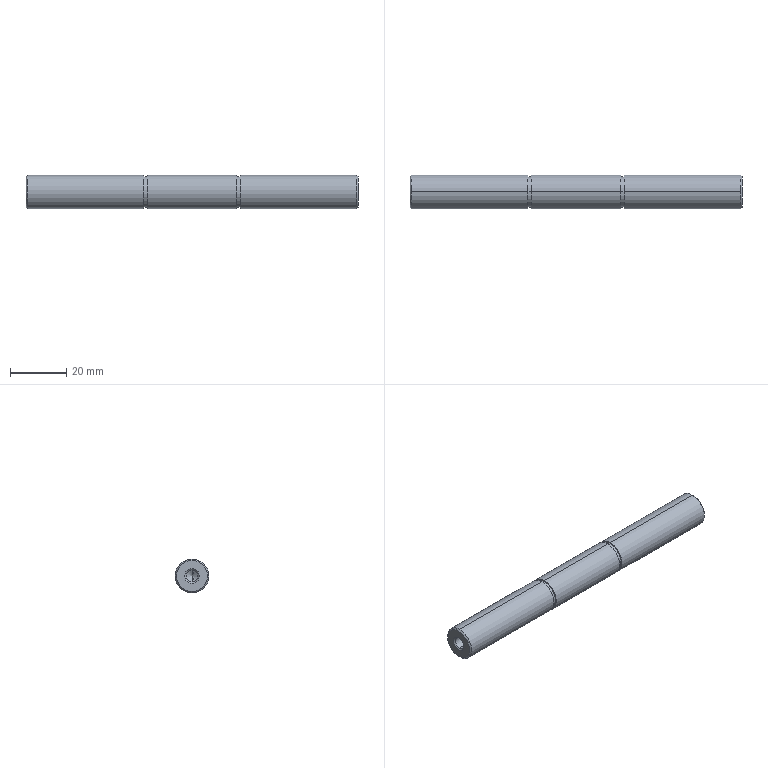Part | SolidWorks | features BaseBody 1 | 1 solid | 32 faces | box 118 x 12 x 12 mm | volume 12890 mm3 | cylinder 14 | cone 12 | plane 6 | commonest cylinder face diameters 12 x6 4.2 x4 11 x4
STEP:
#1=CARTESIAN_POINT('',(41.9,0.,6.));
#2=VERTEX_POINT('',#1);
#3=CARTESIAN_POINT('',(41.9,0.,-6.));
#4=VERTEX_POINT('',#3);
#5=CARTESIAN_POINT('',(41.9,0.,0.));
#6=DIRECTION('',(-1.,0.,0.));
#7=DIRECTION('',(0.,0.,1.));
#8=AXIS2_PLACEMENT_3D('',#5,#6,#7);
#9=CIRCLE('',#8,6.);
#10=EDGE_CURVE('',#2,#4,#9,.T.);
#11=ORIENTED_EDGE('',*,*,#10,.T.);
#12=CARTESIAN_POINT('',(0.5,0.,-6.));
#13=VERTEX_POINT('',#12);
#14=CARTESIAN_POINT('',(118.,0.,-6.));
#15=DIRECTION('',(-1.,0.,0.));
#16=VECTOR('',#15,1000.);
#17=LINE('',#14,#16);
#18=EDGE_CURVE('',#4,#13,#17,.T.);
#19=ORIENTED_EDGE('',*,*,#18,.T.);
#20=CARTESIAN_POINT('',(0.5,0.,6.));
#21=VERTEX_POINT('',#20);
#22=CARTESIAN_POINT('',(0.5,0.,0.));
#23=DIRECTION('',(1.,0.,0.));
#24=DIRECTION('',(0.,0.,-1.));
#25=AXIS2_PLACEMENT_3D('',#22,#23,#24);
#26=CIRCLE('',#25,6.);
#27=EDGE_CURVE('',#13,#21,#26,.T.);
#28=ORIENTED_EDGE('',*,*,#27,.T.);
#29=CARTESIAN_POINT('',(118.,0.,6.));
#30=DIRECTION('',(-1.,0.,0.));
#31=VECTOR('',#30,1000.);
#32=LINE('',#29,#31);
#33=EDGE_CURVE('',#2,#21,#32,.T.);
#34=ORIENTED_EDGE('',*,*,#33,.F.);
#35=EDGE_LOOP('',(#11,#19,#28,#34));
#36=FACE_OUTER_BOUND('',#35,.T.);
#37=CARTESIAN_POINT('',(118.,0.,0.));
#38=DIRECTION('',(-1.,0.,0.));
#39=DIRECTION('',(0.,0.,1.));
#40=AXIS2_PLACEMENT_3D('',#37,#38,#39);
#41=CYLINDRICAL_SURFACE('',#40,6.);
#42=ADVANCED_FACE('',(#36),#41,.T.);
#43=CARTESIAN_POINT('',(0.,0.,5.5));
#44=VERTEX_POINT('',#43);
#45=CARTESIAN_POINT('',(0.,0.,-5.5));
#46=VERTEX_POINT('',#45);
#47=CARTESIAN_POINT('',(0.,0.,0.));
#48=DIRECTION('',(-1.,0.,0.));
#49=DIRECTION('',(0.,0.,-1.));
#50=AXIS2_PLACEMENT_3D('',#47,#48,#49);
#51=CIRCLE('',#50,5.5);
#52=EDGE_CURVE('',#44,#46,#51,.T.);
#53=ORIENTED_EDGE('',*,*,#52,.F.);
#54=CARTESIAN_POINT('',(0.5,0.,6.));
#55=DIRECTION('',(0.7071,0.,0.7071));
#56=VECTOR('',#55,1000.);
#57=LINE('',#54,#56);
#58=EDGE_CURVE('',#44,#21,#57,.T.);
#59=ORIENTED_EDGE('',*,*,#58,.T.);
#60=ORIENTED_EDGE('',*,*,#27,.F.);
#61=CARTESIAN_POINT('',(0.5,0.,-6.));
#62=DIRECTION('',(0.7071,0.,-0.7071));
#63=VECTOR('',#62,1000.);
#64=LINE('',#61,#63);
#65=EDGE_CURVE('',#46,#13,#64,.T.);
#66=ORIENTED_EDGE('',*,*,#65,.F.);
#67=EDGE_LOOP('',(#53,#59,#60,#66));
#68=FACE_OUTER_BOUND('',#67,.T.);
#69=CARTESIAN_POINT('',(0.5,0.,0.));
#70=DIRECTION('',(1.,0.,0.));
#71=DIRECTION('',(0.,0.,-1.));
#72=AXIS2_PLACEMENT_3D('',#69,#70,#71);
#73=CONICAL_SURFACE('',#72,6.,0.7854);
#74=ADVANCED_FACE('',(#68),#73,.T.);
#75=CARTESIAN_POINT('',(0.5,0.,-2.1));
#76=VERTEX_POINT('',#75);
#77=CARTESIAN_POINT('',(0.5,0.,2.1));
#78=VERTEX_POINT('',#77);
#79=CARTESIAN_POINT('',(0.5,0.,0.));
#80=DIRECTION('',(-1.,0.,0.));
#81=DIRECTION('',(0.,0.,-1.));
#82=AXIS2_PLACEMENT_3D('',#79,#80,#81);
#83=CIRCLE('',#82,2.1);
#84=EDGE_CURVE('',#76,#78,#83,.T.);
#85=ORIENTED_EDGE('',*,*,#84,.F.);
#86=CARTESIAN_POINT('',(0.,0.,-2.6));
#87=VERTEX_POINT('',#86);
#88=CARTESIAN_POINT('',(0.5,0.,-2.1));
#89=DIRECTION('',(-0.7071,0.,-0.7071));
#90=VECTOR('',#89,1000.);
#91=LINE('',#88,#90);
#92=EDGE_CURVE('',#76,#87,#91,.T.);
#93=ORIENTED_EDGE('',*,*,#92,.T.);
#94=CARTESIAN_POINT('',(0.,0.,2.6));
#95=VERTEX_POINT('',#94);
#96=CARTESIAN_POINT('',(0.,0.,0.));
#97=DIRECTION('',(1.,0.,0.));
#98=DIRECTION('',(0.,0.,-1.));
#99=AXIS2_PLACEMENT_3D('',#96,#97,#98);
#100=CIRCLE('',#99,2.6);
#101=EDGE_CURVE('',#95,#87,#100,.T.);
#102=ORIENTED_EDGE('',*,*,#101,.F.);
#103=CARTESIAN_POINT('',(0.5,0.,2.1));
#104=DIRECTION('',(-0.7071,0.,0.7071));
#105=VECTOR('',#104,1000.);
#106=LINE('',#103,#105);
#107=EDGE_CURVE('',#78,#95,#106,.T.);
#108=ORIENTED_EDGE('',*,*,#107,.F.);
#109=EDGE_LOOP('',(#85,#93,#102,#108));
#110=FACE_OUTER_BOUND('',#109,.T.);
#111=CARTESIAN_POINT('',(0.5,0.,0.));
#112=DIRECTION('',(-1.,0.,0.));
#113=DIRECTION('',(0.,0.,1.));
#114=AXIS2_PLACEMENT_3D('',#111,#112,#113);
#115=CONICAL_SURFACE('',#114,2.1,0.7854);
#116=ADVANCED_FACE('',(#110),#115,.F.);
#117=CARTESIAN_POINT('',(14.,0.,-2.1));
#118=VERTEX_POINT('',#117);
#119=CARTESIAN_POINT('',(14.,0.,2.1));
#120=VERTEX_POINT('',#119);
#121=CARTESIAN_POINT('',(14.,0.,0.));
#122=DIRECTION('',(-1.,0.,0.));
#123=DIRECTION('',(0.,0.,1.));
#124=AXIS2_PLACEMENT_3D('',#121,#122,#123);
#125=CIRCLE('',#124,2.1);
#126=EDGE_CURVE('',#118,#120,#125,.T.);
#127=ORIENTED_EDGE('',*,*,#126,.F.);
#128=CARTESIAN_POINT('',(0.,0.,-2.1));
#129=DIRECTION('',(-1.,0.,0.));
#130=VECTOR('',#129,1000.);
#131=LINE('',#128,#130);
#132=EDGE_CURVE('',#118,#76,#131,.T.);
#133=ORIENTED_EDGE('',*,*,#132,.T.);
#134=ORIENTED_EDGE('',*,*,#84,.T.);
#135=CARTESIAN_POINT('',(0.,0.,2.1));
#136=DIRECTION('',(-1.,0.,0.));
#137=VECTOR('',#136,1000.);
#138=LINE('',#135,#137);
#139=EDGE_CURVE('',#120,#78,#138,.T.);
#140=ORIENTED_EDGE('',*,*,#139,.F.);
#141=EDGE_LOOP('',(#127,#133,#134,#140));
#142=FACE_OUTER_BOUND('',#141,.T.);
#143=CARTESIAN_POINT('',(0.,0.,0.));
#144=DIRECTION('',(-1.,0.,0.));
#145=DIRECTION('',(0.,0.,1.));
#146=AXIS2_PLACEMENT_3D('',#143,#144,#145);
#147=CYLINDRICAL_SURFACE('',#146,2.1);
#148=ADVANCED_FACE('',(#142),#147,.F.);
#149=CARTESIAN_POINT('',(15.262,0.,0.));
#150=VERTEX_POINT('',#149);
#151=CARTESIAN_POINT('',(14.,0.,2.1));
#152=DIRECTION('',(-0.515,0.,0.8572));
#153=VECTOR('',#152,1000.);
#154=LINE('',#151,#153);
#155=EDGE_CURVE('',#150,#120,#154,.T.);
#156=ORIENTED_EDGE('',*,*,#155,.F.);
#157=CARTESIAN_POINT('',(14.,0.,-2.1));
#158=DIRECTION('',(-0.515,0.,-0.8572));
#159=VECTOR('',#158,1000.);
#160=LINE('',#157,#159);
#161=EDGE_CURVE('',#150,#118,#160,.T.);
#162=ORIENTED_EDGE('',*,*,#161,.T.);
#163=ORIENTED_EDGE('',*,*,#126,.T.);
#164=EDGE_LOOP('',(#156,#162,#163));
#165=FACE_OUTER_BOUND('',#164,.T.);
#166=CARTESIAN_POINT('',(14.,0.,0.));
#167=DIRECTION('',(-1.,0.,0.));
#168=DIRECTION('',(0.,0.,1.));
#169=AXIS2_PLACEMENT_3D('',#166,#167,#168);
#170=CONICAL_SURFACE('',#169,2.1,1.03);
#171=ADVANCED_FACE('',(#165),#170,.F.);
#172=CARTESIAN_POINT('',(43.1,0.,5.5));
#173=VERTEX_POINT('',#172);
#174=CARTESIAN_POINT('',(43.1,0.,-5.5));
#175=VERTEX_POINT('',#174);
#176=CARTESIAN_POINT('',(43.1,0.,0.));
#177=DIRECTION('',(-1.,0.,0.));
#178=DIRECTION('',(0.,0.,1.));
#179=AXIS2_PLACEMENT_3D('',#176,#177,#178);
#180=CIRCLE('',#179,5.5);
#181=EDGE_CURVE('',#173,#175,#180,.T.);
#182=ORIENTED_EDGE('',*,*,#181,.T.);
#183=CARTESIAN_POINT('',(41.9,0.,-5.5));
#184=VERTEX_POINT('',#183);
#185=CARTESIAN_POINT('',(0.,0.,-5.5));
#186=DIRECTION('',(-1.,0.,0.));
#187=VECTOR('',#186,1000.);
#188=LINE('',#185,#187);
#189=EDGE_CURVE('',#175,#184,#188,.T.);
#190=ORIENTED_EDGE('',*,*,#189,.T.);
#191=CARTESIAN_POINT('',(41.9,0.,5.5));
#192=VERTEX_POINT('',#191);
#193=CARTESIAN_POINT('',(41.9,0.,0.));
#194=DIRECTION('',(-1.,0.,0.));
#195=DIRECTION('',(0.,0.,1.));
#196=AXIS2_PLACEMENT_3D('',#193,#194,#195);
#197=CIRCLE('',#196,5.5);
#198=EDGE_CURVE('',#192,#184,#197,.T.);
#199=ORIENTED_EDGE('',*,*,#198,.F.);
#200=CARTESIAN_POINT('',(0.,0.,5.5));
#201=DIRECTION('',(-1.,0.,0.));
#202=VECTOR('',#201,1000.);
#203=LINE('',#200,#202);
#204=EDGE_CURVE('',#173,#192,#203,.T.);
#205=ORIENTED_EDGE('',*,*,#204,.F.);
#206=EDGE_LOOP('',(#182,#190,#199,#205));
#207=FACE_OUTER_BOUND('',#206,.T.);
#208=CARTESIAN_POINT('',(0.,0.,0.));
#209=DIRECTION('',(-1.,0.,0.));
#210=DIRECTION('',(0.,0.,1.));
#211=AXIS2_PLACEMENT_3D('',#208,#209,#210);
#212=CYLINDRICAL_SURFACE('',#211,5.5);
#213=ADVANCED_FACE('',(#207),#212,.T.);
#214=CARTESIAN_POINT('',(76.1,0.,5.5));
#215=VERTEX_POINT('',#214);
#216=CARTESIAN_POINT('',(76.1,0.,-5.5));
#217=VERTEX_POINT('',#216);
#218=CARTESIAN_POINT('',(76.1,0.,0.));
#219=DIRECTION('',(-1.,0.,0.));
#220=DIRECTION('',(0.,0.,1.));
#221=AXIS2_PLACEMENT_3D('',#218,#219,#220);
#222=CIRCLE('',#221,5.5);
#223=EDGE_CURVE('',#215,#217,#222,.T.);
#224=ORIENTED_EDGE('',*,*,#223,.T.);
#225=CARTESIAN_POINT('',(74.9,0.,-5.5));
#226=VERTEX_POINT('',#225);
#227=CARTESIAN_POINT('',(0.,0.,-5.5));
#228=DIRECTION('',(-1.,0.,0.));
#229=VECTOR('',#228,1000.);
#230=LINE('',#227,#229);
#231=EDGE_CURVE('',#217,#226,#230,.T.);
#232=ORIENTED_EDGE('',*,*,#231,.T.);
#233=CARTESIAN_POINT('',(74.9,0.,5.5));
#234=VERTEX_POINT('',#233);
#235=CARTESIAN_POINT('',(74.9,0.,0.));
#236=DIRECTION('',(-1.,0.,0.));
#237=DIRECTION('',(0.,0.,1.));
#238=AXIS2_PLACEMENT_3D('',#235,#236,#237);
#239=CIRCLE('',#238,5.5);
#240=EDGE_CURVE('',#234,#226,#239,.T.);
#241=ORIENTED_EDGE('',*,*,#240,.F.);
#242=CARTESIAN_POINT('',(0.,0.,5.5));
#243=DIRECTION('',(-1.,0.,0.));
#244=VECTOR('',#243,1000.);
#245=LINE('',#242,#244);
#246=EDGE_CURVE('',#215,#234,#245,.T.);
#247=ORIENTED_EDGE('',*,*,#246,.F.);
#248=EDGE_LOOP('',(#224,#232,#241,#247));
#249=FACE_OUTER_BOUND('',#248,.T.);
#250=CARTESIAN_POINT('',(0.,0.,0.));
#251=DIRECTION('',(-1.,0.,0.));
#252=DIRECTION('',(0.,0.,1.));
#253=AXIS2_PLACEMENT_3D('',#250,#251,#252);
#254=CYLINDRICAL_SURFACE('',#253,5.5);
#255=ADVANCED_FACE('',(#249),#254,.T.);
#256=CARTESIAN_POINT('',(117.5,0.,2.1));
#257=VERTEX_POINT('',#256);
#258=CARTESIAN_POINT('',(117.5,0.,-2.1));
#259=VERTEX_POINT('',#258);
#260=CARTESIAN_POINT('',(117.5,0.,0.));
#261=DIRECTION('',(1.,0.,0.));
#262=DIRECTION('',(0.,0.,-1.));
#263=AXIS2_PLACEMENT_3D('',#260,#261,#262);
#264=CIRCLE('',#263,2.1);
#265=EDGE_CURVE('',#257,#259,#264,.T.);
#266=ORIENTED_EDGE('',*,*,#265,.F.);
#267=CARTESIAN_POINT('',(118.,0.,2.6));
#268=VERTEX_POINT('',#267);
#269=CARTESIAN_POINT('',(117.5,0.,2.1));
#270=DIRECTION('',(0.7071,0.,0.7071));
#271=VECTOR('',#270,1000.);
#272=LINE('',#269,#271);
#273=EDGE_CURVE('',#257,#268,#272,.T.);
#274=ORIENTED_EDGE('',*,*,#273,.T.);
#275=CARTESIAN_POINT('',(118.,0.,-2.6));
#276=VERTEX_POINT('',#275);
#277=CARTESIAN_POINT('',(118.,0.,0.));
#278=DIRECTION('',(-1.,0.,0.));
#279=DIRECTION('',(0.,0.,-1.));
#280=AXIS2_PLACEMENT_3D('',#277,#278,#279);
#281=CIRCLE('',#280,2.6);
#282=EDGE_CURVE('',#276,#268,#281,.T.);
#283=ORIENTED_EDGE('',*,*,#282,.F.);
#284=CARTESIAN_POINT('',(117.5,0.,-2.1));
#285=DIRECTION('',(0.7071,0.,-0.7071));
#286=VECTOR('',#285,1000.);
#287=LINE('',#284,#286);
#288=EDGE_CURVE('',#259,#276,#287,.T.);
#289=ORIENTED_EDGE('',*,*,#288,.F.);
#290=EDGE_LOOP('',(#266,#274,#283,#289));
#291=FACE_OUTER_BOUND('',#290,.T.);
#292=CARTESIAN_POINT('',(117.5,0.,0.));
#293=DIRECTION('',(1.,0.,0.));
#294=DIRECTION('',(0.,0.,-1.));
#295=AXIS2_PLACEMENT_3D('',#292,#293,#294);
#296=CONICAL_SURFACE('',#295,2.1,0.7854);
#297=ADVANCED_FACE('',(#291),#296,.F.);
#298=CARTESIAN_POINT('',(118.,0.,-5.5));
#299=VERTEX_POINT('',#298);
#300=CARTESIAN_POINT('',(118.,0.,5.5));
#301=VERTEX_POINT('',#300);
#302=CARTESIAN_POINT('',(118.,0.,0.));
#303=DIRECTION('',(1.,0.,0.));
#304=DIRECTION('',(0.,0.,-1.));
#305=AXIS2_PLACEMENT_3D('',#302,#303,#304);
#306=CIRCLE('',#305,5.5);
#307=EDGE_CURVE('',#299,#301,#306,.T.);
#308=ORIENTED_EDGE('',*,*,#307,.F.);
#309=CARTESIAN_POINT('',(117.5,0.,-6.));
#310=VERTEX_POINT('',#309);
#311=CARTESIAN_POINT('',(118.,0.,-5.5));
#312=DIRECTION('',(-0.7071,0.,-0.7071));
#313=VECTOR('',#312,1000.);
#314=LINE('',#311,#313);
#315=EDGE_CURVE('',#299,#310,#314,.T.);
#316=ORIENTED_EDGE('',*,*,#315,.T.);
#317=CARTESIAN_POINT('',(117.5,0.,6.));
#318=VERTEX_POINT('',#317);
#319=CARTESIAN_POINT('',(117.5,0.,0.));
#320=DIRECTION('',(-1.,0.,0.));
#321=DIRECTION('',(0.,0.,-1.));
#322=AXIS2_PLACEMENT_3D('',#319,#320,#321);
#323=CIRCLE('',#322,6.);
#324=EDGE_CURVE('',#318,#310,#323,.T.);
#325=ORIENTED_EDGE('',*,*,#324,.F.);
#326=CARTESIAN_POINT('',(118.,0.,5.5));
#327=DIRECTION('',(-0.7071,0.,0.7071));
#328=VECTOR('',#327,1000.);
#329=LINE('',#326,#328);
#330=EDGE_CURVE('',#301,#318,#329,.T.);
#331=ORIENTED_EDGE('',*,*,#330,.F.);
#332=EDGE_LOOP('',(#308,#316,#325,#331));
#333=FACE_OUTER_BOUND('',#332,.T.);
#334=CARTESIAN_POINT('',(118.,0.,0.));
#335=DIRECTION('',(-1.,0.,0.));
#336=DIRECTION('',(0.,0.,1.));
#337=AXIS2_PLACEMENT_3D('',#334,#335,#336);
#338=CONICAL_SURFACE('',#337,5.5,0.7854);
#339=ADVANCED_FACE('',(#333),#338,.T.);
#340=CARTESIAN_POINT('',(104.,0.,2.1));
#341=VERTEX_POINT('',#340);
#342=CARTESIAN_POINT('',(104.,0.,-2.1));
#343=VERTEX_POINT('',#342);
#344=CARTESIAN_POINT('',(104.,0.,0.));
#345=DIRECTION('',(1.,0.,0.));
#346=DIRECTION('',(0.,0.,-1.));
#347=AXIS2_PLACEMENT_3D('',#344,#345,#346);
#348=CIRCLE('',#347,2.1);
#349=EDGE_CURVE('',#341,#343,#348,.T.);
#350=ORIENTED_EDGE('',*,*,#349,.F.);
#351=CARTESIAN_POINT('',(118.,0.,2.1));
#352=DIRECTION('',(1.,0.,0.));
#353=VECTOR('',#352,1000.);
#354=LINE('',#351,#353);
#355=EDGE_CURVE('',#341,#257,#354,.T.);
#356=ORIENTED_EDGE('',*,*,#355,.T.);
#357=ORIENTED_EDGE('',*,*,#265,.T.);
#358=CARTESIAN_POINT('',(118.,0.,-2.1));
#359=DIRECTION('',(1.,0.,0.));
#360=VECTOR('',#359,1000.);
#361=LINE('',#358,#360);
#362=EDGE_CURVE('',#343,#259,#361,.T.);
#363=ORIENTED_EDGE('',*,*,#362,.F.);
#364=EDGE_LOOP('',(#350,#356,#357,#363));
#365=FACE_OUTER_BOUND('',#364,.T.);
#366=CARTESIAN_POINT('',(118.,0.,0.));
#367=DIRECTION('',(1.,0.,0.));
#368=DIRECTION('',(0.,0.,-1.));
#369=AXIS2_PLACEMENT_3D('',#366,#367,#368);
#370=CYLINDRICAL_SURFACE('',#369,2.1);
#371=ADVANCED_FACE('',(#365),#370,.F.);
#372=CARTESIAN_POINT('',(102.738,0.,0.));
#373=VERTEX_POINT('',#372);
#374=CARTESIAN_POINT('',(104.,0.,-2.1));
#375=DIRECTION('',(0.515,0.,-0.8572));
#376=VECTOR('',#375,1000.);
#377=LINE('',#374,#376);
#378=EDGE_CURVE('',#373,#343,#377,.T.);
#379=ORIENTED_EDGE('',*,*,#378,.F.);
#380=CARTESIAN_POINT('',(104.,0.,2.1));
#381=DIRECTION('',(0.515,0.,0.8572));
#382=VECTOR('',#381,1000.);
#383=LINE('',#380,#382);
#384=EDGE_CURVE('',#373,#341,#383,.T.);
#385=ORIENTED_EDGE('',*,*,#384,.T.);
#386=ORIENTED_EDGE('',*,*,#349,.T.);
#387=EDGE_LOOP('',(#379,#385,#386));
#388=FACE_OUTER_BOUND('',#387,.T.);
#389=CARTESIAN_POINT('',(104.,0.,0.));
#390=DIRECTION('',(1.,0.,0.));
#391=DIRECTION('',(0.,0.,-1.));
#392=AXIS2_PLACEMENT_3D('',#389,#390,#391);
#393=CONICAL_SURFACE('',#392,2.1,1.03);
#394=ADVANCED_FACE('',(#388),#393,.F.);
#395=ORIENTED_EDGE('',*,*,#324,.T.);
#396=CARTESIAN_POINT('',(76.1,0.,-6.));
#397=VERTEX_POINT('',#396);
#398=CARTESIAN_POINT('',(118.,0.,-6.));
#399=DIRECTION('',(-1.,0.,0.));
#400=VECTOR('',#399,1000.);
#401=LINE('',#398,#400);
#402=EDGE_CURVE('',#310,#397,#401,.T.);
#403=ORIENTED_EDGE('',*,*,#402,.T.);
#404=CARTESIAN_POINT('',(76.1,0.,6.));
#405=VERTEX_POINT('',#404);
#406=CARTESIAN_POINT('',(76.1,0.,0.));
#407=DIRECTION('',(1.,0.,0.));
#408=DIRECTION('',(0.,0.,-1.));
#409=AXIS2_PLACEMENT_3D('',#406,#407,#408);
#410=CIRCLE('',#409,6.);
#411=EDGE_CURVE('',#397,#405,#410,.T.);
#412=ORIENTED_EDGE('',*,*,#411,.T.);
#413=CARTESIAN_POINT('',(118.,0.,6.));
#414=DIRECTION('',(-1.,0.,0.));
#415=VECTOR('',#414,1000.);
#416=LINE('',#413,#415);
#417=EDGE_CURVE('',#318,#405,#416,.T.);
#418=ORIENTED_EDGE('',*,*,#417,.F.);
#419=EDGE_LOOP('',(#395,#403,#412,#418));
#420=FACE_OUTER_BOUND('',#419,.T.);
#421=CARTESIAN_POINT('',(118.,0.,0.));
#422=DIRECTION('',(-1.,0.,0.));
#423=DIRECTION('',(0.,0.,1.));
#424=AXIS2_PLACEMENT_3D('',#421,#422,#423);
#425=CYLINDRICAL_SURFACE('',#424,6.);
#426=ADVANCED_FACE('',(#420),#425,.T.);
#427=CARTESIAN_POINT('',(74.9,0.,6.));
#428=VERTEX_POINT('',#427);
#429=CARTESIAN_POINT('',(74.9,0.,-6.));
#430=VERTEX_POINT('',#429);
#431=CARTESIAN_POINT('',(74.9,0.,0.));
#432=DIRECTION('',(-1.,0.,0.));
#433=DIRECTION('',(0.,0.,1.));
#434=AXIS2_PLACEMENT_3D('',#431,#432,#433);
#435=CIRCLE('',#434,6.);
#436=EDGE_CURVE('',#428,#430,#435,.T.);
#437=ORIENTED_EDGE('',*,*,#436,.T.);
#438=CARTESIAN_POINT('',(43.1,0.,-6.));
#439=VERTEX_POINT('',#438);
#440=CARTESIAN_POINT('',(118.,0.,-6.));
#441=DIRECTION('',(-1.,0.,0.));
#442=VECTOR('',#441,1000.);
#443=LINE('',#440,#442);
#444=EDGE_CURVE('',#430,#439,#443,.T.);
#445=ORIENTED_EDGE('',*,*,#444,.T.);
#446=CARTESIAN_POINT('',(43.1,0.,6.));
#447=VERTEX_POINT('',#446);
#448=CARTESIAN_POINT('',(43.1,0.,0.));
#449=DIRECTION('',(1.,0.,0.));
#450=DIRECTION('',(0.,0.,-1.));
#451=AXIS2_PLACEMENT_3D('',#448,#449,#450);
#452=CIRCLE('',#451,6.);
#453=EDGE_CURVE('',#439,#447,#452,.T.);
#454=ORIENTED_EDGE('',*,*,#453,.T.);
#455=CARTESIAN_POINT('',(118.,0.,6.));
#456=DIRECTION('',(-1.,0.,0.));
#457=VECTOR('',#456,1000.);
#458=LINE('',#455,#457);
#459=EDGE_CURVE('',#428,#447,#458,.T.);
#460=ORIENTED_EDGE('',*,*,#459,.F.);
#461=EDGE_LOOP('',(#437,#445,#454,#460));
#462=FACE_OUTER_BOUND('',#461,.T.);
#463=CARTESIAN_POINT('',(118.,0.,0.));
#464=DIRECTION('',(-1.,0.,0.));
#465=DIRECTION('',(0.,0.,1.));
#466=AXIS2_PLACEMENT_3D('',#463,#464,#465);
#467=CYLINDRICAL_SURFACE('',#466,6.);
#468=ADVANCED_FACE('',(#462),#467,.T.);
#469=ORIENTED_EDGE('',*,*,#444,.F.);
#470=CARTESIAN_POINT('',(74.9,0.,0.));
#471=DIRECTION('',(-1.,0.,0.));
#472=DIRECTION('',(0.,0.,1.));
#473=AXIS2_PLACEMENT_3D('',#470,#471,#472);
#474=CIRCLE('',#473,6.);
#475=EDGE_CURVE('',#430,#428,#474,.T.);
#476=ORIENTED_EDGE('',*,*,#475,.T.);
#477=ORIENTED_EDGE('',*,*,#459,.T.);
#478=CARTESIAN_POINT('',(43.1,0.,0.));
#479=DIRECTION('',(1.,0.,0.));
#480=DIRECTION('',(0.,0.,-1.));
#481=AXIS2_PLACEMENT_3D('',#478,#479,#480);
#482=CIRCLE('',#481,6.);
#483=EDGE_CURVE('',#447,#439,#482,.T.);
#484=ORIENTED_EDGE('',*,*,#483,.T.);
#485=EDGE_LOOP('',(#469,#476,#477,#484));
#486=FACE_OUTER_BOUND('',#485,.T.);
#487=CARTESIAN_POINT('',(118.,0.,0.));
#488=DIRECTION('',(-1.,0.,0.));
#489=DIRECTION('',(0.,0.,1.));
#490=AXIS2_PLACEMENT_3D('',#487,#488,#489);
#491=CYLINDRICAL_SURFACE('',#490,6.);
#492=ADVANCED_FACE('',(#486),#491,.T.);
#493=ORIENTED_EDGE('',*,*,#402,.F.);
#494=CARTESIAN_POINT('',(117.5,0.,0.));
#495=DIRECTION('',(-1.,0.,0.));
#496=DIRECTION('',(0.,0.,-1.));
#497=AXIS2_PLACEMENT_3D('',#494,#495,#496);
#498=CIRCLE('',#497,6.);
#499=EDGE_CURVE('',#310,#318,#498,.T.);
#500=ORIENTED_EDGE('',*,*,#499,.T.);
#501=ORIENTED_EDGE('',*,*,#417,.T.);
#502=CARTESIAN_POINT('',(76.1,0.,0.));
#503=DIRECTION('',(1.,0.,0.));
#504=DIRECTION('',(0.,0.,-1.));
#505=AXIS2_PLACEMENT_3D('',#502,#503,#504);
#506=CIRCLE('',#505,6.);
#507=EDGE_CURVE('',#405,#397,#506,.T.);
#508=ORIENTED_EDGE('',*,*,#507,.T.);
#509=EDGE_LOOP('',(#493,#500,#501,#508));
#510=FACE_OUTER_BOUND('',#509,.T.);
#511=CARTESIAN_POINT('',(118.,0.,0.));
#512=DIRECTION('',(-1.,0.,0.));
#513=DIRECTION('',(0.,0.,1.));
#514=AXIS2_PLACEMENT_3D('',#511,#512,#513);
#515=CYLINDRICAL_SURFACE('',#514,6.);
#516=ADVANCED_FACE('',(#510),#515,.T.);
#517=CARTESIAN_POINT('',(118.,0.,0.));
#518=DIRECTION('',(1.,0.,0.));
#519=DIRECTION('',(0.,0.,-1.));
#520=AXIS2_PLACEMENT_3D('',#517,#518,#519);
#521=CIRCLE('',#520,5.5);
#522=EDGE_CURVE('',#301,#299,#521,.T.);
#523=ORIENTED_EDGE('',*,*,#522,.T.);
#524=ORIENTED_EDGE('',*,*,#307,.T.);
#525=EDGE_LOOP('',(#523,#524));
#526=FACE_OUTER_BOUND('',#525,.T.);
#527=ORIENTED_EDGE('',*,*,#282,.T.);
#528=CARTESIAN_POINT('',(118.,0.,0.));
#529=DIRECTION('',(-1.,0.,0.));
#530=DIRECTION('',(0.,0.,-1.));
#531=AXIS2_PLACEMENT_3D('',#528,#529,#530);
#532=CIRCLE('',#531,2.6);
#533=EDGE_CURVE('',#268,#276,#532,.T.);
#534=ORIENTED_EDGE('',*,*,#533,.T.);
#535=EDGE_LOOP('',(#527,#534));
#536=FACE_BOUND('',#535,.T.);
#537=CARTESIAN_POINT('',(118.,0.,0.));
#538=DIRECTION('',(1.,0.,0.));
#539=DIRECTION('',(0.,0.,-1.));
#540=AXIS2_PLACEMENT_3D('',#537,#538,#539);
#541=PLANE('',#540);
#542=ADVANCED_FACE('',(#526,#536),#541,.T.);
#543=ORIENTED_EDGE('',*,*,#384,.F.);
#544=ORIENTED_EDGE('',*,*,#378,.T.);
#545=CARTESIAN_POINT('',(104.,0.,0.));
#546=DIRECTION('',(1.,0.,0.));
#547=DIRECTION('',(0.,0.,-1.));
#548=AXIS2_PLACEMENT_3D('',#545,#546,#547);
#549=CIRCLE('',#548,2.1);
#550=EDGE_CURVE('',#343,#341,#549,.T.);
#551=ORIENTED_EDGE('',*,*,#550,.T.);
#552=EDGE_LOOP('',(#543,#544,#551));
#553=FACE_OUTER_BOUND('',#552,.T.);
#554=CARTESIAN_POINT('',(104.,0.,0.));
#555=DIRECTION('',(1.,0.,0.));
#556=DIRECTION('',(0.,0.,-1.));
#557=AXIS2_PLACEMENT_3D('',#554,#555,#556);
#558=CONICAL_SURFACE('',#557,2.1,1.03);
#559=ADVANCED_FACE('',(#553),#558,.F.);
#560=ORIENTED_EDGE('',*,*,#355,.F.);
#561=ORIENTED_EDGE('',*,*,#550,.F.);
#562=ORIENTED_EDGE('',*,*,#362,.T.);
#563=CARTESIAN_POINT('',(117.5,0.,0.));
#564=DIRECTION('',(1.,0.,0.));
#565=DIRECTION('',(0.,0.,-1.));
#566=AXIS2_PLACEMENT_3D('',#563,#564,#565);
#567=CIRCLE('',#566,2.1);
#568=EDGE_CURVE('',#259,#257,#567,.T.);
#569=ORIENTED_EDGE('',*,*,#568,.T.);
#570=EDGE_LOOP('',(#560,#561,#562,#569));
#571=FACE_OUTER_BOUND('',#570,.T.);
#572=CARTESIAN_POINT('',(118.,0.,0.));
#573=DIRECTION('',(1.,0.,0.));
#574=DIRECTION('',(0.,0.,-1.));
#575=AXIS2_PLACEMENT_3D('',#572,#573,#574);
#576=CYLINDRICAL_SURFACE('',#575,2.1);
#577=ADVANCED_FACE('',(#571),#576,.F.);
#578=ORIENTED_EDGE('',*,*,#315,.F.);
#579=ORIENTED_EDGE('',*,*,#522,.F.);
#580=ORIENTED_EDGE('',*,*,#330,.T.);
#581=ORIENTED_EDGE('',*,*,#499,.F.);
#582=EDGE_LOOP('',(#578,#579,#580,#581));
#583=FACE_OUTER_BOUND('',#582,.T.);
#584=CARTESIAN_POINT('',(118.,0.,0.));
#585=DIRECTION('',(-1.,0.,0.));
#586=DIRECTION('',(0.,0.,1.));
#587=AXIS2_PLACEMENT_3D('',#584,#585,#586);
#588=CONICAL_SURFACE('',#587,5.5,0.7854);
#589=ADVANCED_FACE('',(#583),#588,.T.);
#590=ORIENTED_EDGE('',*,*,#273,.F.);
#591=ORIENTED_EDGE('',*,*,#568,.F.);
#592=ORIENTED_EDGE('',*,*,#288,.T.);
#593=ORIENTED_EDGE('',*,*,#533,.F.);
#594=EDGE_LOOP('',(#590,#591,#592,#593));
#595=FACE_OUTER_BOUND('',#594,.T.);
#596=CARTESIAN_POINT('',(117.5,0.,0.));
#597=DIRECTION('',(1.,0.,0.));
#598=DIRECTION('',(0.,0.,-1.));
#599=AXIS2_PLACEMENT_3D('',#596,#597,#598);
#600=CONICAL_SURFACE('',#599,2.1,0.7854);
#601=ADVANCED_FACE('',(#595),#600,.F.);
#602=ORIENTED_EDGE('',*,*,#223,.F.);
#603=CARTESIAN_POINT('',(76.1,0.,0.));
#604=DIRECTION('',(-1.,0.,0.));
#605=DIRECTION('',(0.,0.,1.));
#606=AXIS2_PLACEMENT_3D('',#603,#604,#605);
#607=CIRCLE('',#606,5.5);
#608=EDGE_CURVE('',#217,#215,#607,.T.);
#609=ORIENTED_EDGE('',*,*,#608,.F.);
#610=EDGE_LOOP('',(#602,#609));
#611=FACE_BOUND('',#610,.T.);
#612=ORIENTED_EDGE('',*,*,#507,.F.);
#613=ORIENTED_EDGE('',*,*,#411,.F.);
#614=EDGE_LOOP('',(#612,#613));
#615=FACE_OUTER_BOUND('',#614,.T.);
#616=CARTESIAN_POINT('',(76.1,-10.5,0.));
#617=DIRECTION('',(1.,0.,0.));
#618=DIRECTION('',(0.,0.,-1.));
#619=AXIS2_PLACEMENT_3D('',#616,#617,#618);
#620=PLANE('',#619);
#621=ADVANCED_FACE('',(#611,#615),#620,.F.);
#622=ORIENTED_EDGE('',*,*,#240,.T.);
#623=CARTESIAN_POINT('',(74.9,0.,0.));
#624=DIRECTION('',(-1.,0.,0.));
#625=DIRECTION('',(0.,0.,1.));
#626=AXIS2_PLACEMENT_3D('',#623,#624,#625);
#627=CIRCLE('',#626,5.5);
#628=EDGE_CURVE('',#226,#234,#627,.T.);
#629=ORIENTED_EDGE('',*,*,#628,.T.);
#630=EDGE_LOOP('',(#622,#629));
#631=FACE_BOUND('',#630,.T.);
#632=ORIENTED_EDGE('',*,*,#436,.F.);
#633=ORIENTED_EDGE('',*,*,#475,.F.);
#634=EDGE_LOOP('',(#632,#633));
#635=FACE_OUTER_BOUND('',#634,.T.);
#636=CARTESIAN_POINT('',(74.9,-10.5,0.));
#637=DIRECTION('',(-1.,0.,0.));
#638=DIRECTION('',(0.,0.,1.));
#639=AXIS2_PLACEMENT_3D('',#636,#637,#638);
#640=PLANE('',#639);
#641=ADVANCED_FACE('',(#631,#635),#640,.F.);
#642=ORIENTED_EDGE('',*,*,#231,.F.);
#643=ORIENTED_EDGE('',*,*,#608,.T.);
#644=ORIENTED_EDGE('',*,*,#246,.T.);
#645=ORIENTED_EDGE('',*,*,#628,.F.);
#646=EDGE_LOOP('',(#642,#643,#644,#645));
#647=FACE_OUTER_BOUND('',#646,.T.);
#648=CARTESIAN_POINT('',(0.,0.,0.));
#649=DIRECTION('',(-1.,0.,0.));
#650=DIRECTION('',(0.,0.,1.));
#651=AXIS2_PLACEMENT_3D('',#648,#649,#650);
#652=CYLINDRICAL_SURFACE('',#651,5.5);
#653=ADVANCED_FACE('',(#647),#652,.T.);
#654=ORIENTED_EDGE('',*,*,#181,.F.);
#655=CARTESIAN_POINT('',(43.1,0.,0.));
#656=DIRECTION('',(-1.,0.,0.));
#657=DIRECTION('',(0.,0.,1.));
#658=AXIS2_PLACEMENT_3D('',#655,#656,#657);
#659=CIRCLE('',#658,5.5);
#660=EDGE_CURVE('',#175,#173,#659,.T.);
#661=ORIENTED_EDGE('',*,*,#660,.F.);
#662=EDGE_LOOP('',(#654,#661));
#663=FACE_BOUND('',#662,.T.);
#664=ORIENTED_EDGE('',*,*,#483,.F.);
#665=ORIENTED_EDGE('',*,*,#453,.F.);
#666=EDGE_LOOP('',(#664,#665));
#667=FACE_OUTER_BOUND('',#666,.T.);
#668=CARTESIAN_POINT('',(43.1,-10.5,0.));
#669=DIRECTION('',(1.,0.,0.));
#670=DIRECTION('',(0.,0.,-1.));
#671=AXIS2_PLACEMENT_3D('',#668,#669,#670);
#672=PLANE('',#671);
#673=ADVANCED_FACE('',(#663,#667),#672,.F.);
#674=ORIENTED_EDGE('',*,*,#198,.T.);
#675=CARTESIAN_POINT('',(41.9,0.,0.));
#676=DIRECTION('',(-1.,0.,0.));
#677=DIRECTION('',(0.,0.,1.));
#678=AXIS2_PLACEMENT_3D('',#675,#676,#677);
#679=CIRCLE('',#678,5.5);
#680=EDGE_CURVE('',#184,#192,#679,.T.);
#681=ORIENTED_EDGE('',*,*,#680,.T.);
#682=EDGE_LOOP('',(#674,#681));
#683=FACE_BOUND('',#682,.T.);
#684=ORIENTED_EDGE('',*,*,#10,.F.);
#685=CARTESIAN_POINT('',(41.9,0.,0.));
#686=DIRECTION('',(-1.,0.,0.));
#687=DIRECTION('',(0.,0.,1.));
#688=AXIS2_PLACEMENT_3D('',#685,#686,#687);
#689=CIRCLE('',#688,6.);
#690=EDGE_CURVE('',#4,#2,#689,.T.);
#691=ORIENTED_EDGE('',*,*,#690,.F.);
#692=EDGE_LOOP('',(#684,#691));
#693=FACE_OUTER_BOUND('',#692,.T.);
#694=CARTESIAN_POINT('',(41.9,-10.5,0.));
#695=DIRECTION('',(-1.,0.,0.));
#696=DIRECTION('',(0.,0.,1.));
#697=AXIS2_PLACEMENT_3D('',#694,#695,#696);
#698=PLANE('',#697);
#699=ADVANCED_FACE('',(#683,#693),#698,.F.);
#700=ORIENTED_EDGE('',*,*,#189,.F.);
#701=ORIENTED_EDGE('',*,*,#660,.T.);
#702=ORIENTED_EDGE('',*,*,#204,.T.);
#703=ORIENTED_EDGE('',*,*,#680,.F.);
#704=EDGE_LOOP('',(#700,#701,#702,#703));
#705=FACE_OUTER_BOUND('',#704,.T.);
#706=CARTESIAN_POINT('',(0.,0.,0.));
#707=DIRECTION('',(-1.,0.,0.));
#708=DIRECTION('',(0.,0.,1.));
#709=AXIS2_PLACEMENT_3D('',#706,#707,#708);
#710=CYLINDRICAL_SURFACE('',#709,5.5);
#711=ADVANCED_FACE('',(#705),#710,.T.);
#712=ORIENTED_EDGE('',*,*,#161,.F.);
#713=ORIENTED_EDGE('',*,*,#155,.T.);
#714=CARTESIAN_POINT('',(14.,0.,0.));
#715=DIRECTION('',(-1.,0.,0.));
#716=DIRECTION('',(0.,0.,1.));
#717=AXIS2_PLACEMENT_3D('',#714,#715,#716);
#718=CIRCLE('',#717,2.1);
#719=EDGE_CURVE('',#120,#118,#718,.T.);
#720=ORIENTED_EDGE('',*,*,#719,.T.);
#721=EDGE_LOOP('',(#712,#713,#720));
#722=FACE_OUTER_BOUND('',#721,.T.);
#723=CARTESIAN_POINT('',(14.,0.,0.));
#724=DIRECTION('',(-1.,0.,0.));
#725=DIRECTION('',(0.,0.,1.));
#726=AXIS2_PLACEMENT_3D('',#723,#724,#725);
#727=CONICAL_SURFACE('',#726,2.1,1.03);
#728=ADVANCED_FACE('',(#722),#727,.F.);
#729=ORIENTED_EDGE('',*,*,#132,.F.);
#730=ORIENTED_EDGE('',*,*,#719,.F.);
#731=ORIENTED_EDGE('',*,*,#139,.T.);
#732=CARTESIAN_POINT('',(0.5,0.,0.));
#733=DIRECTION('',(-1.,0.,0.));
#734=DIRECTION('',(0.,0.,-1.));
#735=AXIS2_PLACEMENT_3D('',#732,#733,#734);
#736=CIRCLE('',#735,2.1);
#737=EDGE_CURVE('',#78,#76,#736,.T.);
#738=ORIENTED_EDGE('',*,*,#737,.T.);
#739=EDGE_LOOP('',(#729,#730,#731,#738));
#740=FACE_OUTER_BOUND('',#739,.T.);
#741=CARTESIAN_POINT('',(0.,0.,0.));
#742=DIRECTION('',(-1.,0.,0.));
#743=DIRECTION('',(0.,0.,1.));
#744=AXIS2_PLACEMENT_3D('',#741,#742,#743);
#745=CYLINDRICAL_SURFACE('',#744,2.1);
#746=ADVANCED_FACE('',(#740),#745,.F.);
#747=ORIENTED_EDGE('',*,*,#92,.F.);
#748=ORIENTED_EDGE('',*,*,#737,.F.);
#749=ORIENTED_EDGE('',*,*,#107,.T.);
#750=CARTESIAN_POINT('',(0.,0.,0.));
#751=DIRECTION('',(1.,0.,0.));
#752=DIRECTION('',(0.,0.,-1.));
#753=AXIS2_PLACEMENT_3D('',#750,#751,#752);
#754=CIRCLE('',#753,2.6);
#755=EDGE_CURVE('',#87,#95,#754,.T.);
#756=ORIENTED_EDGE('',*,*,#755,.F.);
#757=EDGE_LOOP('',(#747,#748,#749,#756));
#758=FACE_OUTER_BOUND('',#757,.T.);
#759=CARTESIAN_POINT('',(0.5,0.,0.));
#760=DIRECTION('',(-1.,0.,0.));
#761=DIRECTION('',(0.,0.,1.));
#762=AXIS2_PLACEMENT_3D('',#759,#760,#761);
#763=CONICAL_SURFACE('',#762,2.1,0.7854);
#764=ADVANCED_FACE('',(#758),#763,.F.);
#765=CARTESIAN_POINT('',(0.,0.,0.));
#766=DIRECTION('',(-1.,0.,0.));
#767=DIRECTION('',(0.,0.,-1.));
#768=AXIS2_PLACEMENT_3D('',#765,#766,#767);
#769=CIRCLE('',#768,5.5);
#770=EDGE_CURVE('',#46,#44,#769,.T.);
#771=ORIENTED_EDGE('',*,*,#770,.T.);
#772=ORIENTED_EDGE('',*,*,#52,.T.);
#773=EDGE_LOOP('',(#771,#772));
#774=FACE_OUTER_BOUND('',#773,.T.);
#775=ORIENTED_EDGE('',*,*,#101,.T.);
#776=ORIENTED_EDGE('',*,*,#755,.T.);
#777=EDGE_LOOP('',(#775,#776));
#778=FACE_BOUND('',#777,.T.);
#779=CARTESIAN_POINT('',(0.,0.,0.));
#780=DIRECTION('',(1.,0.,0.));
#781=DIRECTION('',(0.,0.,-1.));
#782=AXIS2_PLACEMENT_3D('',#779,#780,#781);
#783=PLANE('',#782);
#784=ADVANCED_FACE('',(#774,#778),#783,.F.);
#785=ORIENTED_EDGE('',*,*,#58,.F.);
#786=ORIENTED_EDGE('',*,*,#770,.F.);
#787=ORIENTED_EDGE('',*,*,#65,.T.);
#788=CARTESIAN_POINT('',(0.5,0.,0.));
#789=DIRECTION('',(1.,0.,0.));
#790=DIRECTION('',(0.,0.,-1.));
#791=AXIS2_PLACEMENT_3D('',#788,#789,#790);
#792=CIRCLE('',#791,6.);
#793=EDGE_CURVE('',#21,#13,#792,.T.);
#794=ORIENTED_EDGE('',*,*,#793,.F.);
#795=EDGE_LOOP('',(#785,#786,#787,#794));
#796=FACE_OUTER_BOUND('',#795,.T.);
#797=CARTESIAN_POINT('',(0.5,0.,0.));
#798=DIRECTION('',(1.,0.,0.));
#799=DIRECTION('',(0.,0.,-1.));
#800=AXIS2_PLACEMENT_3D('',#797,#798,#799);
#801=CONICAL_SURFACE('',#800,6.,0.7854);
#802=ADVANCED_FACE('',(#796),#801,.T.);
#803=ORIENTED_EDGE('',*,*,#18,.F.);
#804=ORIENTED_EDGE('',*,*,#690,.T.);
#805=ORIENTED_EDGE('',*,*,#33,.T.);
#806=ORIENTED_EDGE('',*,*,#793,.T.);
#807=EDGE_LOOP('',(#803,#804,#805,#806));
#808=FACE_OUTER_BOUND('',#807,.T.);
#809=CARTESIAN_POINT('',(118.,0.,0.));
#810=DIRECTION('',(-1.,0.,0.));
#811=DIRECTION('',(0.,0.,1.));
#812=AXIS2_PLACEMENT_3D('',#809,#810,#811);
#813=CYLINDRICAL_SURFACE('',#812,6.);
#814=ADVANCED_FACE('',(#808),#813,.T.);
#815=CLOSED_SHELL('',(#42,#74,#116,#148,#171,#213,#255,#297,#339,#371,#394,#426,#468,#492,#516,#542,#559,#577,#589,#601,#621,#641,#653,#673,#699,#711,#728,#746,#764,#784,#802,#814));
#816=MANIFOLD_SOLID_BREP('',#815);
#817=CARTESIAN_POINT('',(0.,0.,0.));
#818=DIRECTION('',(0.,0.,1.));
#819=DIRECTION('',(1.,0.,0.));
#820=AXIS2_PLACEMENT_3D('',#817,#818,#819);
#821=(LENGTH_UNIT()NAMED_UNIT(*)SI_UNIT(.MILLI.,.METRE.));
#822=UNCERTAINTY_MEASURE_WITH_UNIT(LENGTH_MEASURE(0.00001),#821,'','');
#823=(NAMED_UNIT(*)PLANE_ANGLE_UNIT()SI_UNIT($,.RADIAN.));
#824=(NAMED_UNIT(*)SI_UNIT($,.STERADIAN.)SOLID_ANGLE_UNIT());
#825=(GEOMETRIC_REPRESENTATION_CONTEXT(3)GLOBAL_UNCERTAINTY_ASSIGNED_CONTEXT((#822))GLOBAL_UNIT_ASSIGNED_CONTEXT((#821,#823,#824))REPRESENTATION_CONTEXT('',''));
#826=ADVANCED_BREP_SHAPE_REPRESENTATION('',(#816,#820),#825);